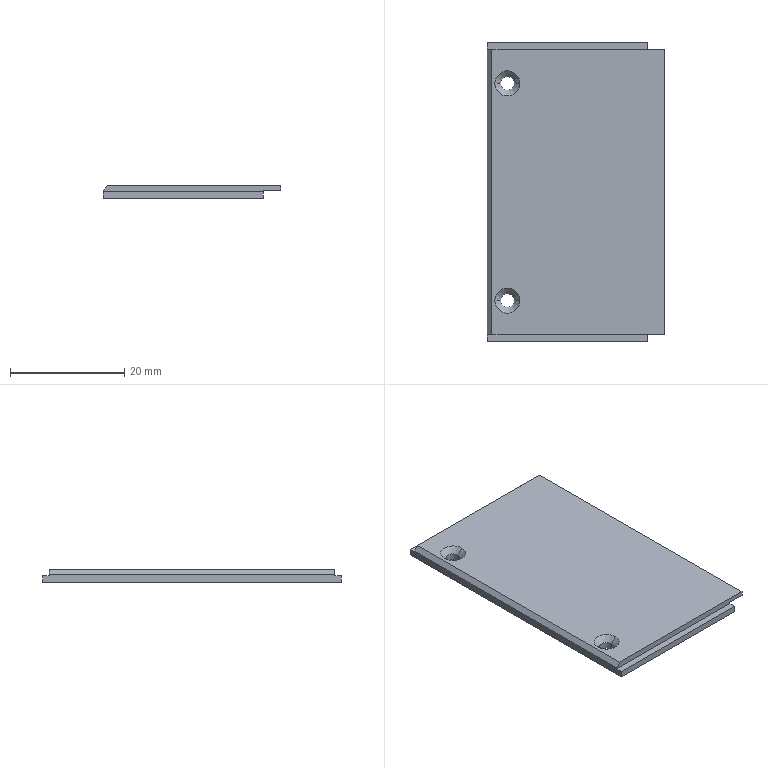Part | STEP file | ASND-0110-OPT-CO60-X-V1.0 upper cover plate | 1 solid | 21 faces | box 31 x 52.3 x 2.2 mm | volume 3229 mm3 | plane 13 | cone 4 | cylinder 4 | commonest cylinder face diameters 2.4 x4